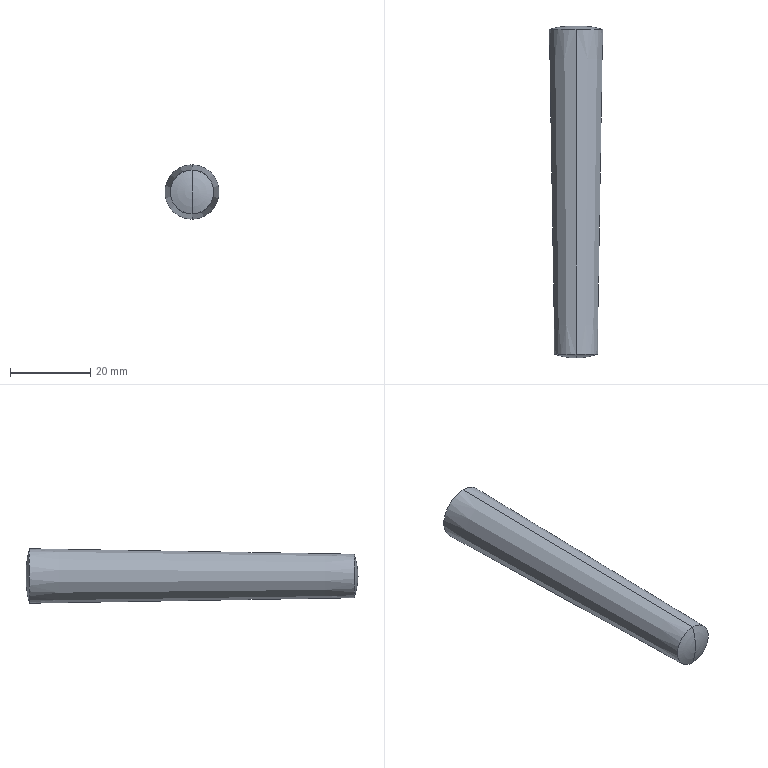Part | SolidWorks | features Revolution 1, Scale 1 | 1 solid | 6 faces | box 13.56 x 82.779 x 13.56 mm | volume 9630 mm3 | torus 4 | cone 2
STEP:
#1=CARTESIAN_POINT('',(0.,-26.494,-5.43));
#2=VERTEX_POINT('',#1);
#3=CARTESIAN_POINT('',(0.,-26.494,5.43));
#4=VERTEX_POINT('',#3);
#5=CARTESIAN_POINT('',(0.,-26.494,0.));
#6=DIRECTION('',(0.,-1.,0.));
#7=DIRECTION('',(0.,0.,-1.));
#8=AXIS2_PLACEMENT_3D('',#5,#6,#7);
#9=CIRCLE('',#8,5.43);
#10=EDGE_CURVE('',#2,#4,#9,.T.);
#11=ORIENTED_EDGE('',*,*,#10,.T.);
#12=CARTESIAN_POINT('',(0.,-27.421,0.));
#13=VERTEX_POINT('',#12);
#14=CARTESIAN_POINT('',(0.,-8.903,-0.3658));
#15=DIRECTION('',(1.,0.,0.));
#16=DIRECTION('',(0.,0.,-1.));
#17=AXIS2_PLACEMENT_3D('',#14,#15,#16);
#18=CIRCLE('',#17,18.521);
#19=EDGE_CURVE('',#4,#13,#18,.T.);
#20=ORIENTED_EDGE('',*,*,#19,.T.);
#21=CARTESIAN_POINT('',(0.,-8.903,0.3658));
#22=DIRECTION('',(-1.,0.,0.));
#23=DIRECTION('',(0.,0.,1.));
#24=AXIS2_PLACEMENT_3D('',#21,#22,#23);
#25=CIRCLE('',#24,18.521);
#26=EDGE_CURVE('',#2,#13,#25,.T.);
#27=ORIENTED_EDGE('',*,*,#26,.F.);
#28=EDGE_LOOP('',(#11,#20,#27));
#29=FACE_OUTER_BOUND('',#28,.T.);
#30=CARTESIAN_POINT('',(0.,-8.903,0.));
#31=DIRECTION('',(0.,-1.,0.));
#32=DIRECTION('',(0.,0.,-1.));
#33=AXIS2_PLACEMENT_3D('',#30,#31,#32);
#34=TOROIDAL_SURFACE('',#33,-0.3658,18.521);
#35=ADVANCED_FACE('',(#29),#34,.T.);
#36=ORIENTED_EDGE('',*,*,#10,.F.);
#37=CARTESIAN_POINT('',(0.,54.508,-6.78));
#38=VERTEX_POINT('',#37);
#39=CARTESIAN_POINT('',(0.,54.508,-6.78));
#40=DIRECTION('',(0.,0.9999,-0.01666));
#41=VECTOR('',#40,1000.);
#42=LINE('',#39,#41);
#43=EDGE_CURVE('',#2,#38,#42,.T.);
#44=ORIENTED_EDGE('',*,*,#43,.T.);
#45=CARTESIAN_POINT('',(0.,54.508,6.78));
#46=VERTEX_POINT('',#45);
#47=CARTESIAN_POINT('',(0.,54.508,0.));
#48=DIRECTION('',(0.,-1.,0.));
#49=DIRECTION('',(0.,0.,-1.));
#50=AXIS2_PLACEMENT_3D('',#47,#48,#49);
#51=CIRCLE('',#50,6.78);
#52=EDGE_CURVE('',#38,#46,#51,.T.);
#53=ORIENTED_EDGE('',*,*,#52,.T.);
#54=CARTESIAN_POINT('',(0.,54.508,6.78));
#55=DIRECTION('',(0.,0.9999,0.01666));
#56=VECTOR('',#55,1000.);
#57=LINE('',#54,#56);
#58=EDGE_CURVE('',#4,#46,#57,.T.);
#59=ORIENTED_EDGE('',*,*,#58,.F.);
#60=EDGE_LOOP('',(#36,#44,#53,#59));
#61=FACE_OUTER_BOUND('',#60,.T.);
#62=CARTESIAN_POINT('',(0.,54.508,0.));
#63=DIRECTION('',(0.,1.,0.));
#64=DIRECTION('',(0.,0.,1.));
#65=AXIS2_PLACEMENT_3D('',#62,#63,#64);
#66=CONICAL_SURFACE('',#65,6.78,0.01667);
#67=ADVANCED_FACE('',(#61),#66,.T.);
#68=CARTESIAN_POINT('',(0.,55.353,0.));
#69=VERTEX_POINT('',#68);
#70=CARTESIAN_POINT('',(0.,31.855,-0.5134));
#71=DIRECTION('',(-1.,0.,0.));
#72=DIRECTION('',(0.,0.,1.));
#73=AXIS2_PLACEMENT_3D('',#70,#71,#72);
#74=CIRCLE('',#73,23.504);
#75=EDGE_CURVE('',#69,#38,#74,.T.);
#76=ORIENTED_EDGE('',*,*,#75,.F.);
#77=CARTESIAN_POINT('',(0.,31.855,0.5134));
#78=DIRECTION('',(1.,0.,0.));
#79=DIRECTION('',(0.,0.,-1.));
#80=AXIS2_PLACEMENT_3D('',#77,#78,#79);
#81=CIRCLE('',#80,23.504);
#82=EDGE_CURVE('',#69,#46,#81,.T.);
#83=ORIENTED_EDGE('',*,*,#82,.T.);
#84=ORIENTED_EDGE('',*,*,#52,.F.);
#85=EDGE_LOOP('',(#76,#83,#84));
#86=FACE_OUTER_BOUND('',#85,.T.);
#87=CARTESIAN_POINT('',(0.,31.855,0.));
#88=DIRECTION('',(0.,-1.,0.));
#89=DIRECTION('',(0.,0.,-1.));
#90=AXIS2_PLACEMENT_3D('',#87,#88,#89);
#91=TOROIDAL_SURFACE('',#90,0.5134,23.504);
#92=ADVANCED_FACE('',(#86),#91,.T.);
#93=ORIENTED_EDGE('',*,*,#82,.F.);
#94=ORIENTED_EDGE('',*,*,#75,.T.);
#95=CARTESIAN_POINT('',(0.,54.508,0.));
#96=DIRECTION('',(0.,-1.,0.));
#97=DIRECTION('',(0.,0.,-1.));
#98=AXIS2_PLACEMENT_3D('',#95,#96,#97);
#99=CIRCLE('',#98,6.78);
#100=EDGE_CURVE('',#46,#38,#99,.T.);
#101=ORIENTED_EDGE('',*,*,#100,.F.);
#102=EDGE_LOOP('',(#93,#94,#101));
#103=FACE_OUTER_BOUND('',#102,.T.);
#104=CARTESIAN_POINT('',(0.,31.855,0.));
#105=DIRECTION('',(0.,-1.,0.));
#106=DIRECTION('',(0.,0.,-1.));
#107=AXIS2_PLACEMENT_3D('',#104,#105,#106);
#108=TOROIDAL_SURFACE('',#107,0.5134,23.504);
#109=ADVANCED_FACE('',(#103),#108,.T.);
#110=ORIENTED_EDGE('',*,*,#43,.F.);
#111=CARTESIAN_POINT('',(0.,-26.494,0.));
#112=DIRECTION('',(0.,-1.,0.));
#113=DIRECTION('',(0.,0.,-1.));
#114=AXIS2_PLACEMENT_3D('',#111,#112,#113);
#115=CIRCLE('',#114,5.43);
#116=EDGE_CURVE('',#4,#2,#115,.T.);
#117=ORIENTED_EDGE('',*,*,#116,.F.);
#118=ORIENTED_EDGE('',*,*,#58,.T.);
#119=ORIENTED_EDGE('',*,*,#100,.T.);
#120=EDGE_LOOP('',(#110,#117,#118,#119));
#121=FACE_OUTER_BOUND('',#120,.T.);
#122=CARTESIAN_POINT('',(0.,54.508,0.));
#123=DIRECTION('',(0.,1.,0.));
#124=DIRECTION('',(0.,0.,1.));
#125=AXIS2_PLACEMENT_3D('',#122,#123,#124);
#126=CONICAL_SURFACE('',#125,6.78,0.01667);
#127=ADVANCED_FACE('',(#121),#126,.T.);
#128=ORIENTED_EDGE('',*,*,#19,.F.);
#129=ORIENTED_EDGE('',*,*,#116,.T.);
#130=ORIENTED_EDGE('',*,*,#26,.T.);
#131=EDGE_LOOP('',(#128,#129,#130));
#132=FACE_OUTER_BOUND('',#131,.T.);
#133=CARTESIAN_POINT('',(0.,-8.903,0.));
#134=DIRECTION('',(0.,-1.,0.));
#135=DIRECTION('',(0.,0.,-1.));
#136=AXIS2_PLACEMENT_3D('',#133,#134,#135);
#137=TOROIDAL_SURFACE('',#136,-0.3658,18.521);
#138=ADVANCED_FACE('',(#132),#137,.T.);
#139=CLOSED_SHELL('',(#35,#67,#92,#109,#127,#138));
#140=MANIFOLD_SOLID_BREP('',#139);
#141=CARTESIAN_POINT('',(0.,0.,0.));
#142=DIRECTION('',(0.,0.,1.));
#143=DIRECTION('',(1.,0.,0.));
#144=AXIS2_PLACEMENT_3D('',#141,#142,#143);
#145=(LENGTH_UNIT()NAMED_UNIT(*)SI_UNIT(.MILLI.,.METRE.));
#146=UNCERTAINTY_MEASURE_WITH_UNIT(LENGTH_MEASURE(0.00001),#145,'','');
#147=(NAMED_UNIT(*)PLANE_ANGLE_UNIT()SI_UNIT($,.RADIAN.));
#148=(NAMED_UNIT(*)SI_UNIT($,.STERADIAN.)SOLID_ANGLE_UNIT());
#149=(GEOMETRIC_REPRESENTATION_CONTEXT(3)GLOBAL_UNCERTAINTY_ASSIGNED_CONTEXT((#146))GLOBAL_UNIT_ASSIGNED_CONTEXT((#145,#147,#148))REPRESENTATION_CONTEXT('',''));
#150=ADVANCED_BREP_SHAPE_REPRESENTATION('',(#140,#144),#149);